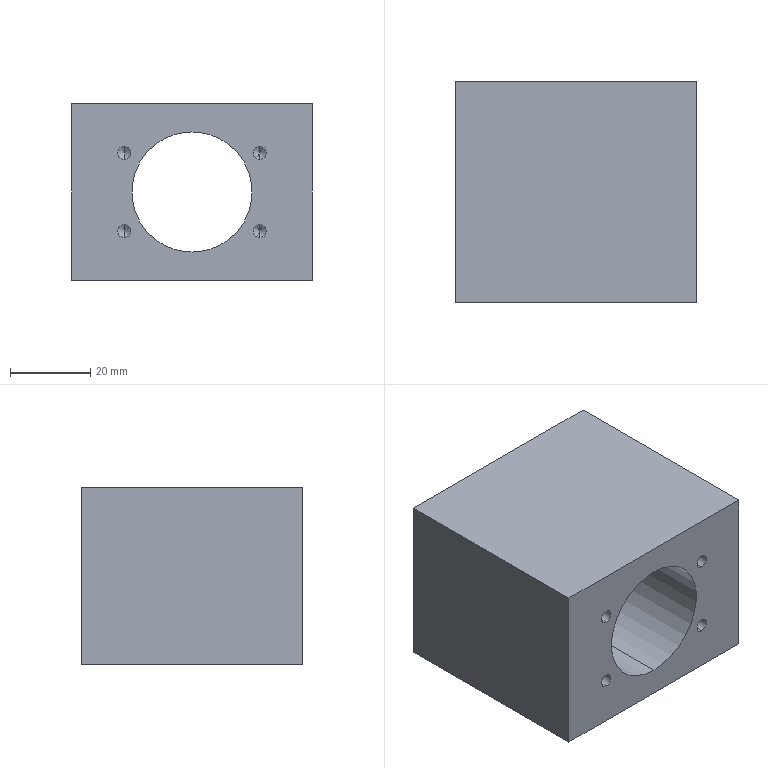Part | STEP file | X77-07003 | 1 solid | 40 faces | box 60 x 55 x 44 mm | volume 104749 mm3 | cylinder 18 | cone 16 | plane 6 | commonest cylinder face diameters 3.3 x8 5 x8 30 x2
STEP:
#1=CARTESIAN_POINT('',(18.182,-106.098,3.));
#2=VERTEX_POINT('',#1);
#3=CARTESIAN_POINT('',(13.182,-106.098,3.));
#4=VERTEX_POINT('',#3);
#5=CARTESIAN_POINT('',(15.682,-106.098,3.));
#6=DIRECTION('',(0.,0.,-1.));
#7=DIRECTION('',(-1.,0.,0.));
#8=AXIS2_PLACEMENT_3D('',#5,#6,#7);
#9=CIRCLE('',#8,2.5);
#10=EDGE_CURVE('',#2,#4,#9,.T.);
#11=ORIENTED_EDGE('',*,*,#10,.F.);
#12=CARTESIAN_POINT('',(18.182,-106.098,-12.));
#13=VERTEX_POINT('',#12);
#14=CARTESIAN_POINT('',(18.182,-106.098,-12.));
#15=DIRECTION('',(0.,0.,-1.));
#16=VECTOR('',#15,1000.);
#17=LINE('',#14,#16);
#18=EDGE_CURVE('',#2,#13,#17,.T.);
#19=ORIENTED_EDGE('',*,*,#18,.T.);
#20=CARTESIAN_POINT('',(13.182,-106.098,-12.));
#21=VERTEX_POINT('',#20);
#22=CARTESIAN_POINT('',(15.682,-106.098,-12.));
#23=DIRECTION('',(0.,0.,-1.));
#24=DIRECTION('',(-1.,0.,0.));
#25=AXIS2_PLACEMENT_3D('',#22,#23,#24);
#26=CIRCLE('',#25,2.5);
#27=EDGE_CURVE('',#13,#21,#26,.T.);
#28=ORIENTED_EDGE('',*,*,#27,.T.);
#29=CARTESIAN_POINT('',(13.182,-106.098,-12.));
#30=DIRECTION('',(0.,0.,-1.));
#31=VECTOR('',#30,1000.);
#32=LINE('',#29,#31);
#33=EDGE_CURVE('',#4,#21,#32,.T.);
#34=ORIENTED_EDGE('',*,*,#33,.F.);
#35=EDGE_LOOP('',(#11,#19,#28,#34));
#36=FACE_OUTER_BOUND('',#35,.T.);
#37=CARTESIAN_POINT('',(15.682,-106.098,-12.));
#38=DIRECTION('',(0.,0.,-1.));
#39=DIRECTION('',(-1.,0.,0.));
#40=AXIS2_PLACEMENT_3D('',#37,#38,#39);
#41=CYLINDRICAL_SURFACE('',#40,2.5);
#42=ADVANCED_FACE('',(#36),#41,.F.);
#43=CARTESIAN_POINT('',(15.682,-106.098,4.502));
#44=VERTEX_POINT('',#43);
#45=CARTESIAN_POINT('',(13.182,-106.098,3.));
#46=DIRECTION('',(-0.8572,0.,-0.515));
#47=VECTOR('',#46,1000.);
#48=LINE('',#45,#47);
#49=EDGE_CURVE('',#44,#4,#48,.T.);
#50=ORIENTED_EDGE('',*,*,#49,.F.);
#51=CARTESIAN_POINT('',(18.182,-106.098,3.));
#52=DIRECTION('',(0.8572,0.,-0.515));
#53=VECTOR('',#52,1000.);
#54=LINE('',#51,#53);
#55=EDGE_CURVE('',#44,#2,#54,.T.);
#56=ORIENTED_EDGE('',*,*,#55,.T.);
#57=ORIENTED_EDGE('',*,*,#10,.T.);
#58=EDGE_LOOP('',(#50,#56,#57));
#59=FACE_OUTER_BOUND('',#58,.T.);
#60=CARTESIAN_POINT('',(15.682,-106.098,3.));
#61=DIRECTION('',(0.,0.,-1.));
#62=DIRECTION('',(-1.,0.,0.));
#63=AXIS2_PLACEMENT_3D('',#60,#61,#62);
#64=CONICAL_SURFACE('',#63,2.5,1.03);
#65=ADVANCED_FACE('',(#59),#64,.F.);
#66=CARTESIAN_POINT('',(-26.818,-106.098,3.));
#67=VERTEX_POINT('',#66);
#68=CARTESIAN_POINT('',(-31.818,-106.098,3.));
#69=VERTEX_POINT('',#68);
#70=CARTESIAN_POINT('',(-29.318,-106.098,3.));
#71=DIRECTION('',(0.,0.,-1.));
#72=DIRECTION('',(-1.,0.,0.));
#73=AXIS2_PLACEMENT_3D('',#70,#71,#72);
#74=CIRCLE('',#73,2.5);
#75=EDGE_CURVE('',#67,#69,#74,.T.);
#76=ORIENTED_EDGE('',*,*,#75,.F.);
#77=CARTESIAN_POINT('',(-26.818,-106.098,-12.));
#78=VERTEX_POINT('',#77);
#79=CARTESIAN_POINT('',(-26.818,-106.098,-12.));
#80=DIRECTION('',(0.,0.,-1.));
#81=VECTOR('',#80,1000.);
#82=LINE('',#79,#81);
#83=EDGE_CURVE('',#67,#78,#82,.T.);
#84=ORIENTED_EDGE('',*,*,#83,.T.);
#85=CARTESIAN_POINT('',(-31.818,-106.098,-12.));
#86=VERTEX_POINT('',#85);
#87=CARTESIAN_POINT('',(-29.318,-106.098,-12.));
#88=DIRECTION('',(0.,0.,-1.));
#89=DIRECTION('',(-1.,0.,0.));
#90=AXIS2_PLACEMENT_3D('',#87,#88,#89);
#91=CIRCLE('',#90,2.5);
#92=EDGE_CURVE('',#78,#86,#91,.T.);
#93=ORIENTED_EDGE('',*,*,#92,.T.);
#94=CARTESIAN_POINT('',(-31.818,-106.098,-12.));
#95=DIRECTION('',(0.,0.,-1.));
#96=VECTOR('',#95,1000.);
#97=LINE('',#94,#96);
#98=EDGE_CURVE('',#69,#86,#97,.T.);
#99=ORIENTED_EDGE('',*,*,#98,.F.);
#100=EDGE_LOOP('',(#76,#84,#93,#99));
#101=FACE_OUTER_BOUND('',#100,.T.);
#102=CARTESIAN_POINT('',(-29.318,-106.098,-12.));
#103=DIRECTION('',(0.,0.,-1.));
#104=DIRECTION('',(-1.,0.,0.));
#105=AXIS2_PLACEMENT_3D('',#102,#103,#104);
#106=CYLINDRICAL_SURFACE('',#105,2.5);
#107=ADVANCED_FACE('',(#101),#106,.F.);
#108=CARTESIAN_POINT('',(-29.318,-106.098,4.502));
#109=VERTEX_POINT('',#108);
#110=CARTESIAN_POINT('',(-31.818,-106.098,3.));
#111=DIRECTION('',(-0.8572,0.,-0.515));
#112=VECTOR('',#111,1000.);
#113=LINE('',#110,#112);
#114=EDGE_CURVE('',#109,#69,#113,.T.);
#115=ORIENTED_EDGE('',*,*,#114,.F.);
#116=CARTESIAN_POINT('',(-26.818,-106.098,3.));
#117=DIRECTION('',(0.8572,0.,-0.515));
#118=VECTOR('',#117,1000.);
#119=LINE('',#116,#118);
#120=EDGE_CURVE('',#109,#67,#119,.T.);
#121=ORIENTED_EDGE('',*,*,#120,.T.);
#122=ORIENTED_EDGE('',*,*,#75,.T.);
#123=EDGE_LOOP('',(#115,#121,#122));
#124=FACE_OUTER_BOUND('',#123,.T.);
#125=CARTESIAN_POINT('',(-29.318,-106.098,3.));
#126=DIRECTION('',(0.,0.,-1.));
#127=DIRECTION('',(-1.,0.,0.));
#128=AXIS2_PLACEMENT_3D('',#125,#126,#127);
#129=CONICAL_SURFACE('',#128,2.5,1.03);
#130=ADVANCED_FACE('',(#124),#129,.F.);
#131=CARTESIAN_POINT('',(18.182,-146.098,3.));
#132=VERTEX_POINT('',#131);
#133=CARTESIAN_POINT('',(13.182,-146.098,3.));
#134=VERTEX_POINT('',#133);
#135=CARTESIAN_POINT('',(15.682,-146.098,3.));
#136=DIRECTION('',(0.,0.,-1.));
#137=DIRECTION('',(-1.,0.,0.));
#138=AXIS2_PLACEMENT_3D('',#135,#136,#137);
#139=CIRCLE('',#138,2.5);
#140=EDGE_CURVE('',#132,#134,#139,.T.);
#141=ORIENTED_EDGE('',*,*,#140,.F.);
#142=CARTESIAN_POINT('',(18.182,-146.098,-12.));
#143=VERTEX_POINT('',#142);
#144=CARTESIAN_POINT('',(18.182,-146.098,-12.));
#145=DIRECTION('',(0.,0.,-1.));
#146=VECTOR('',#145,1000.);
#147=LINE('',#144,#146);
#148=EDGE_CURVE('',#132,#143,#147,.T.);
#149=ORIENTED_EDGE('',*,*,#148,.T.);
#150=CARTESIAN_POINT('',(13.182,-146.098,-12.));
#151=VERTEX_POINT('',#150);
#152=CARTESIAN_POINT('',(15.682,-146.098,-12.));
#153=DIRECTION('',(0.,0.,-1.));
#154=DIRECTION('',(-1.,0.,0.));
#155=AXIS2_PLACEMENT_3D('',#152,#153,#154);
#156=CIRCLE('',#155,2.5);
#157=EDGE_CURVE('',#143,#151,#156,.T.);
#158=ORIENTED_EDGE('',*,*,#157,.T.);
#159=CARTESIAN_POINT('',(13.182,-146.098,-12.));
#160=DIRECTION('',(0.,0.,-1.));
#161=VECTOR('',#160,1000.);
#162=LINE('',#159,#161);
#163=EDGE_CURVE('',#134,#151,#162,.T.);
#164=ORIENTED_EDGE('',*,*,#163,.F.);
#165=EDGE_LOOP('',(#141,#149,#158,#164));
#166=FACE_OUTER_BOUND('',#165,.T.);
#167=CARTESIAN_POINT('',(15.682,-146.098,-12.));
#168=DIRECTION('',(0.,0.,-1.));
#169=DIRECTION('',(-1.,0.,0.));
#170=AXIS2_PLACEMENT_3D('',#167,#168,#169);
#171=CYLINDRICAL_SURFACE('',#170,2.5);
#172=ADVANCED_FACE('',(#166),#171,.F.);
#173=CARTESIAN_POINT('',(15.682,-146.098,4.502));
#174=VERTEX_POINT('',#173);
#175=CARTESIAN_POINT('',(13.182,-146.098,3.));
#176=DIRECTION('',(-0.8572,0.,-0.515));
#177=VECTOR('',#176,1000.);
#178=LINE('',#175,#177);
#179=EDGE_CURVE('',#174,#134,#178,.T.);
#180=ORIENTED_EDGE('',*,*,#179,.F.);
#181=CARTESIAN_POINT('',(18.182,-146.098,3.));
#182=DIRECTION('',(0.8572,0.,-0.515));
#183=VECTOR('',#182,1000.);
#184=LINE('',#181,#183);
#185=EDGE_CURVE('',#174,#132,#184,.T.);
#186=ORIENTED_EDGE('',*,*,#185,.T.);
#187=ORIENTED_EDGE('',*,*,#140,.T.);
#188=EDGE_LOOP('',(#180,#186,#187));
#189=FACE_OUTER_BOUND('',#188,.T.);
#190=CARTESIAN_POINT('',(15.682,-146.098,3.));
#191=DIRECTION('',(0.,0.,-1.));
#192=DIRECTION('',(-1.,0.,0.));
#193=AXIS2_PLACEMENT_3D('',#190,#191,#192);
#194=CONICAL_SURFACE('',#193,2.5,1.03);
#195=ADVANCED_FACE('',(#189),#194,.F.);
#196=CARTESIAN_POINT('',(-26.818,-146.098,3.));
#197=VERTEX_POINT('',#196);
#198=CARTESIAN_POINT('',(-31.818,-146.098,3.));
#199=VERTEX_POINT('',#198);
#200=CARTESIAN_POINT('',(-29.318,-146.098,3.));
#201=DIRECTION('',(0.,0.,-1.));
#202=DIRECTION('',(-1.,0.,0.));
#203=AXIS2_PLACEMENT_3D('',#200,#201,#202);
#204=CIRCLE('',#203,2.5);
#205=EDGE_CURVE('',#197,#199,#204,.T.);
#206=ORIENTED_EDGE('',*,*,#205,.F.);
#207=CARTESIAN_POINT('',(-26.818,-146.098,-12.));
#208=VERTEX_POINT('',#207);
#209=CARTESIAN_POINT('',(-26.818,-146.098,-12.));
#210=DIRECTION('',(0.,0.,-1.));
#211=VECTOR('',#210,1000.);
#212=LINE('',#209,#211);
#213=EDGE_CURVE('',#197,#208,#212,.T.);
#214=ORIENTED_EDGE('',*,*,#213,.T.);
#215=CARTESIAN_POINT('',(-31.818,-146.098,-12.));
#216=VERTEX_POINT('',#215);
#217=CARTESIAN_POINT('',(-29.318,-146.098,-12.));
#218=DIRECTION('',(0.,0.,-1.));
#219=DIRECTION('',(-1.,0.,0.));
#220=AXIS2_PLACEMENT_3D('',#217,#218,#219);
#221=CIRCLE('',#220,2.5);
#222=EDGE_CURVE('',#208,#216,#221,.T.);
#223=ORIENTED_EDGE('',*,*,#222,.T.);
#224=CARTESIAN_POINT('',(-31.818,-146.098,-12.));
#225=DIRECTION('',(0.,0.,-1.));
#226=VECTOR('',#225,1000.);
#227=LINE('',#224,#226);
#228=EDGE_CURVE('',#199,#216,#227,.T.);
#229=ORIENTED_EDGE('',*,*,#228,.F.);
#230=EDGE_LOOP('',(#206,#214,#223,#229));
#231=FACE_OUTER_BOUND('',#230,.T.);
#232=CARTESIAN_POINT('',(-29.318,-146.098,-12.));
#233=DIRECTION('',(0.,0.,-1.));
#234=DIRECTION('',(-1.,0.,0.));
#235=AXIS2_PLACEMENT_3D('',#232,#233,#234);
#236=CYLINDRICAL_SURFACE('',#235,2.5);
#237=ADVANCED_FACE('',(#231),#236,.F.);
#238=CARTESIAN_POINT('',(-29.318,-146.098,4.502));
#239=VERTEX_POINT('',#238);
#240=CARTESIAN_POINT('',(-31.818,-146.098,3.));
#241=DIRECTION('',(-0.8572,0.,-0.515));
#242=VECTOR('',#241,1000.);
#243=LINE('',#240,#242);
#244=EDGE_CURVE('',#239,#199,#243,.T.);
#245=ORIENTED_EDGE('',*,*,#244,.F.);
#246=CARTESIAN_POINT('',(-26.818,-146.098,3.));
#247=DIRECTION('',(0.8572,0.,-0.515));
#248=VECTOR('',#247,1000.);
#249=LINE('',#246,#248);
#250=EDGE_CURVE('',#239,#197,#249,.T.);
#251=ORIENTED_EDGE('',*,*,#250,.T.);
#252=ORIENTED_EDGE('',*,*,#205,.T.);
#253=EDGE_LOOP('',(#245,#251,#252));
#254=FACE_OUTER_BOUND('',#253,.T.);
#255=CARTESIAN_POINT('',(-29.318,-146.098,3.));
#256=DIRECTION('',(0.,0.,-1.));
#257=DIRECTION('',(-1.,0.,0.));
#258=AXIS2_PLACEMENT_3D('',#255,#256,#257);
#259=CONICAL_SURFACE('',#258,2.5,1.03);
#260=ADVANCED_FACE('',(#254),#259,.F.);
#261=CARTESIAN_POINT('',(-23.706,-143.498,21.4));
#262=VERTEX_POINT('',#261);
#263=CARTESIAN_POINT('',(-23.706,-143.498,18.1));
#264=VERTEX_POINT('',#263);
#265=CARTESIAN_POINT('',(-23.706,-143.498,19.75));
#266=DIRECTION('',(0.,-1.,0.));
#267=DIRECTION('',(0.,0.,-1.));
#268=AXIS2_PLACEMENT_3D('',#265,#266,#267);
#269=CIRCLE('',#268,1.65);
#270=EDGE_CURVE('',#262,#264,#269,.T.);
#271=ORIENTED_EDGE('',*,*,#270,.F.);
#272=CARTESIAN_POINT('',(-23.706,-153.598,21.4));
#273=VERTEX_POINT('',#272);
#274=CARTESIAN_POINT('',(-23.706,-153.598,21.4));
#275=DIRECTION('',(0.,-1.,0.));
#276=VECTOR('',#275,1000.);
#277=LINE('',#274,#276);
#278=EDGE_CURVE('',#262,#273,#277,.T.);
#279=ORIENTED_EDGE('',*,*,#278,.T.);
#280=CARTESIAN_POINT('',(-23.706,-153.598,18.1));
#281=VERTEX_POINT('',#280);
#282=CARTESIAN_POINT('',(-23.706,-153.598,19.75));
#283=DIRECTION('',(0.,-1.,0.));
#284=DIRECTION('',(0.,0.,-1.));
#285=AXIS2_PLACEMENT_3D('',#282,#283,#284);
#286=CIRCLE('',#285,1.65);
#287=EDGE_CURVE('',#273,#281,#286,.T.);
#288=ORIENTED_EDGE('',*,*,#287,.T.);
#289=CARTESIAN_POINT('',(-23.706,-153.598,18.1));
#290=DIRECTION('',(0.,-1.,0.));
#291=VECTOR('',#290,1000.);
#292=LINE('',#289,#291);
#293=EDGE_CURVE('',#264,#281,#292,.T.);
#294=ORIENTED_EDGE('',*,*,#293,.F.);
#295=EDGE_LOOP('',(#271,#279,#288,#294));
#296=FACE_OUTER_BOUND('',#295,.T.);
#297=CARTESIAN_POINT('',(-23.706,-153.598,19.75));
#298=DIRECTION('',(0.,-1.,0.));
#299=DIRECTION('',(0.,0.,-1.));
#300=AXIS2_PLACEMENT_3D('',#297,#298,#299);
#301=CYLINDRICAL_SURFACE('',#300,1.65);
#302=ADVANCED_FACE('',(#296),#301,.F.);
#303=CARTESIAN_POINT('',(-23.706,-142.506,19.75));
#304=VERTEX_POINT('',#303);
#305=CARTESIAN_POINT('',(-23.706,-143.498,18.1));
#306=DIRECTION('',(0.,-0.515,-0.8572));
#307=VECTOR('',#306,1000.);
#308=LINE('',#305,#307);
#309=EDGE_CURVE('',#304,#264,#308,.T.);
#310=ORIENTED_EDGE('',*,*,#309,.F.);
#311=CARTESIAN_POINT('',(-23.706,-143.498,21.4));
#312=DIRECTION('',(0.,-0.515,0.8572));
#313=VECTOR('',#312,1000.);
#314=LINE('',#311,#313);
#315=EDGE_CURVE('',#304,#262,#314,.T.);
#316=ORIENTED_EDGE('',*,*,#315,.T.);
#317=ORIENTED_EDGE('',*,*,#270,.T.);
#318=EDGE_LOOP('',(#310,#316,#317));
#319=FACE_OUTER_BOUND('',#318,.T.);
#320=CARTESIAN_POINT('',(-23.706,-143.498,19.75));
#321=DIRECTION('',(0.,-1.,0.));
#322=DIRECTION('',(0.,0.,-1.));
#323=AXIS2_PLACEMENT_3D('',#320,#321,#322);
#324=CONICAL_SURFACE('',#323,1.65,1.03);
#325=ADVANCED_FACE('',(#319),#324,.F.);
#326=CARTESIAN_POINT('',(-23.706,-143.498,1.9));
#327=VERTEX_POINT('',#326);
#328=CARTESIAN_POINT('',(-23.706,-143.498,-1.4));
#329=VERTEX_POINT('',#328);
#330=CARTESIAN_POINT('',(-23.706,-143.498,0.25));
#331=DIRECTION('',(0.,-1.,0.));
#332=DIRECTION('',(0.,0.,-1.));
#333=AXIS2_PLACEMENT_3D('',#330,#331,#332);
#334=CIRCLE('',#333,1.65);
#335=EDGE_CURVE('',#327,#329,#334,.T.);
#336=ORIENTED_EDGE('',*,*,#335,.F.);
#337=CARTESIAN_POINT('',(-23.706,-153.598,1.9));
#338=VERTEX_POINT('',#337);
#339=CARTESIAN_POINT('',(-23.706,-153.598,1.9));
#340=DIRECTION('',(0.,-1.,0.));
#341=VECTOR('',#340,1000.);
#342=LINE('',#339,#341);
#343=EDGE_CURVE('',#327,#338,#342,.T.);
#344=ORIENTED_EDGE('',*,*,#343,.T.);
#345=CARTESIAN_POINT('',(-23.706,-153.598,-1.4));
#346=VERTEX_POINT('',#345);
#347=CARTESIAN_POINT('',(-23.706,-153.598,0.25));
#348=DIRECTION('',(0.,-1.,0.));
#349=DIRECTION('',(0.,0.,-1.));
#350=AXIS2_PLACEMENT_3D('',#347,#348,#349);
#351=CIRCLE('',#350,1.65);
#352=EDGE_CURVE('',#338,#346,#351,.T.);
#353=ORIENTED_EDGE('',*,*,#352,.T.);
#354=CARTESIAN_POINT('',(-23.706,-153.598,-1.4));
#355=DIRECTION('',(0.,-1.,0.));
#356=VECTOR('',#355,1000.);
#357=LINE('',#354,#356);
#358=EDGE_CURVE('',#329,#346,#357,.T.);
#359=ORIENTED_EDGE('',*,*,#358,.F.);
#360=EDGE_LOOP('',(#336,#344,#353,#359));
#361=FACE_OUTER_BOUND('',#360,.T.);
#362=CARTESIAN_POINT('',(-23.706,-153.598,0.25));
#363=DIRECTION('',(0.,-1.,0.));
#364=DIRECTION('',(0.,0.,-1.));
#365=AXIS2_PLACEMENT_3D('',#362,#363,#364);
#366=CYLINDRICAL_SURFACE('',#365,1.65);
#367=ADVANCED_FACE('',(#361),#366,.F.);
#368=CARTESIAN_POINT('',(-23.706,-142.506,0.25));
#369=VERTEX_POINT('',#368);
#370=CARTESIAN_POINT('',(-23.706,-143.498,-1.4));
#371=DIRECTION('',(0.,-0.515,-0.8572));
#372=VECTOR('',#371,1000.);
#373=LINE('',#370,#372);
#374=EDGE_CURVE('',#369,#329,#373,.T.);
#375=ORIENTED_EDGE('',*,*,#374,.F.);
#376=CARTESIAN_POINT('',(-23.706,-143.498,1.9));
#377=DIRECTION('',(0.,-0.515,0.8572));
#378=VECTOR('',#377,1000.);
#379=LINE('',#376,#378);
#380=EDGE_CURVE('',#369,#327,#379,.T.);
#381=ORIENTED_EDGE('',*,*,#380,.T.);
#382=ORIENTED_EDGE('',*,*,#335,.T.);
#383=EDGE_LOOP('',(#375,#381,#382));
#384=FACE_OUTER_BOUND('',#383,.T.);
#385=CARTESIAN_POINT('',(-23.706,-143.498,0.25));
#386=DIRECTION('',(0.,-1.,0.));
#387=DIRECTION('',(0.,0.,-1.));
#388=AXIS2_PLACEMENT_3D('',#385,#386,#387);
#389=CONICAL_SURFACE('',#388,1.65,1.03);
#390=ADVANCED_FACE('',(#384),#389,.F.);
#391=CARTESIAN_POINT('',(10.069,-143.498,1.9));
#392=VERTEX_POINT('',#391);
#393=CARTESIAN_POINT('',(10.069,-143.498,-1.4));
#394=VERTEX_POINT('',#393);
#395=CARTESIAN_POINT('',(10.069,-143.498,0.25));
#396=DIRECTION('',(0.,-1.,0.));
#397=DIRECTION('',(0.,0.,-1.));
#398=AXIS2_PLACEMENT_3D('',#395,#396,#397);
#399=CIRCLE('',#398,1.65);
#400=EDGE_CURVE('',#392,#394,#399,.T.);
#401=ORIENTED_EDGE('',*,*,#400,.F.);
#402=CARTESIAN_POINT('',(10.069,-153.598,1.9));
#403=VERTEX_POINT('',#402);
#404=CARTESIAN_POINT('',(10.069,-153.598,1.9));
#405=DIRECTION('',(0.,-1.,0.));
#406=VECTOR('',#405,1000.);
#407=LINE('',#404,#406);
#408=EDGE_CURVE('',#392,#403,#407,.T.);
#409=ORIENTED_EDGE('',*,*,#408,.T.);
#410=CARTESIAN_POINT('',(10.069,-153.598,-1.4));
#411=VERTEX_POINT('',#410);
#412=CARTESIAN_POINT('',(10.069,-153.598,0.25));
#413=DIRECTION('',(0.,-1.,0.));
#414=DIRECTION('',(0.,0.,-1.));
#415=AXIS2_PLACEMENT_3D('',#412,#413,#414);
#416=CIRCLE('',#415,1.65);
#417=EDGE_CURVE('',#403,#411,#416,.T.);
#418=ORIENTED_EDGE('',*,*,#417,.T.);
#419=CARTESIAN_POINT('',(10.069,-153.598,-1.4));
#420=DIRECTION('',(0.,-1.,0.));
#421=VECTOR('',#420,1000.);
#422=LINE('',#419,#421);
#423=EDGE_CURVE('',#394,#411,#422,.T.);
#424=ORIENTED_EDGE('',*,*,#423,.F.);
#425=EDGE_LOOP('',(#401,#409,#418,#424));
#426=FACE_OUTER_BOUND('',#425,.T.);
#427=CARTESIAN_POINT('',(10.069,-153.598,0.25));
#428=DIRECTION('',(0.,-1.,0.));
#429=DIRECTION('',(0.,0.,-1.));
#430=AXIS2_PLACEMENT_3D('',#427,#428,#429);
#431=CYLINDRICAL_SURFACE('',#430,1.65);
#432=ADVANCED_FACE('',(#426),#431,.F.);
#433=CARTESIAN_POINT('',(10.069,-142.506,0.25));
#434=VERTEX_POINT('',#433);
#435=CARTESIAN_POINT('',(10.069,-143.498,-1.4));
#436=DIRECTION('',(0.,-0.515,-0.8572));
#437=VECTOR('',#436,1000.);
#438=LINE('',#435,#437);
#439=EDGE_CURVE('',#434,#394,#438,.T.);
#440=ORIENTED_EDGE('',*,*,#439,.F.);
#441=CARTESIAN_POINT('',(10.069,-143.498,1.9));
#442=DIRECTION('',(0.,-0.515,0.8572));
#443=VECTOR('',#442,1000.);
#444=LINE('',#441,#443);
#445=EDGE_CURVE('',#434,#392,#444,.T.);
#446=ORIENTED_EDGE('',*,*,#445,.T.);
#447=ORIENTED_EDGE('',*,*,#400,.T.);
#448=EDGE_LOOP('',(#440,#446,#447));
#449=FACE_OUTER_BOUND('',#448,.T.);
#450=CARTESIAN_POINT('',(10.069,-143.498,0.25));
#451=DIRECTION('',(0.,-1.,0.));
#452=DIRECTION('',(0.,0.,-1.));
#453=AXIS2_PLACEMENT_3D('',#450,#451,#452);
#454=CONICAL_SURFACE('',#453,1.65,1.03);
#455=ADVANCED_FACE('',(#449),#454,.F.);
#456=CARTESIAN_POINT('',(10.069,-143.498,21.4));
#457=VERTEX_POINT('',#456);
#458=CARTESIAN_POINT('',(10.069,-143.498,18.1));
#459=VERTEX_POINT('',#458);
#460=CARTESIAN_POINT('',(10.069,-143.498,19.75));
#461=DIRECTION('',(0.,-1.,0.));
#462=DIRECTION('',(0.,0.,-1.));
#463=AXIS2_PLACEMENT_3D('',#460,#461,#462);
#464=CIRCLE('',#463,1.65);
#465=EDGE_CURVE('',#457,#459,#464,.T.);
#466=ORIENTED_EDGE('',*,*,#465,.F.);
#467=CARTESIAN_POINT('',(10.069,-153.598,21.4));
#468=VERTEX_POINT('',#467);
#469=CARTESIAN_POINT('',(10.069,-153.598,21.4));
#470=DIRECTION('',(0.,-1.,0.));
#471=VECTOR('',#470,1000.);
#472=LINE('',#469,#471);
#473=EDGE_CURVE('',#457,#468,#472,.T.);
#474=ORIENTED_EDGE('',*,*,#473,.T.);
#475=CARTESIAN_POINT('',(10.069,-153.598,18.1));
#476=VERTEX_POINT('',#475);
#477=CARTESIAN_POINT('',(10.069,-153.598,19.75));
#478=DIRECTION('',(0.,-1.,0.));
#479=DIRECTION('',(0.,0.,-1.));
#480=AXIS2_PLACEMENT_3D('',#477,#478,#479);
#481=CIRCLE('',#480,1.65);
#482=EDGE_CURVE('',#468,#476,#481,.T.);
#483=ORIENTED_EDGE('',*,*,#482,.T.);
#484=CARTESIAN_POINT('',(10.069,-153.598,18.1));
#485=DIRECTION('',(0.,-1.,0.));
#486=VECTOR('',#485,1000.);
#487=LINE('',#484,#486);
#488=EDGE_CURVE('',#459,#476,#487,.T.);
#489=ORIENTED_EDGE('',*,*,#488,.F.);
#490=EDGE_LOOP('',(#466,#474,#483,#489));
#491=FACE_OUTER_BOUND('',#490,.T.);
#492=CARTESIAN_POINT('',(10.069,-153.598,19.75));
#493=DIRECTION('',(0.,-1.,0.));
#494=DIRECTION('',(0.,0.,-1.));
#495=AXIS2_PLACEMENT_3D('',#492,#493,#494);
#496=CYLINDRICAL_SURFACE('',#495,1.65);
#497=ADVANCED_FACE('',(#491),#496,.F.);
#498=CARTESIAN_POINT('',(10.069,-142.506,19.75));
#499=VERTEX_POINT('',#498);
#500=CARTESIAN_POINT('',(10.069,-143.498,18.1));
#501=DIRECTION('',(0.,-0.515,-0.8572));
#502=VECTOR('',#501,1000.);
#503=LINE('',#500,#502);
#504=EDGE_CURVE('',#499,#459,#503,.T.);
#505=ORIENTED_EDGE('',*,*,#504,.F.);
#506=CARTESIAN_POINT('',(10.069,-143.498,21.4));
#507=DIRECTION('',(0.,-0.515,0.8572));
#508=VECTOR('',#507,1000.);
#509=LINE('',#506,#508);
#510=EDGE_CURVE('',#499,#457,#509,.T.);
#511=ORIENTED_EDGE('',*,*,#510,.T.);
#512=ORIENTED_EDGE('',*,*,#465,.T.);
#513=EDGE_LOOP('',(#505,#511,#512));
#514=FACE_OUTER_BOUND('',#513,.T.);
#515=CARTESIAN_POINT('',(10.069,-143.498,19.75));
#516=DIRECTION('',(0.,-1.,0.));
#517=DIRECTION('',(0.,0.,-1.));
#518=AXIS2_PLACEMENT_3D('',#515,#516,#517);
#519=CONICAL_SURFACE('',#518,1.65,1.03);
#520=ADVANCED_FACE('',(#514),#519,.F.);
#521=CARTESIAN_POINT('',(-6.818,-153.598,-5.));
#522=VERTEX_POINT('',#521);
#523=CARTESIAN_POINT('',(-6.818,-153.598,25.));
#524=VERTEX_POINT('',#523);
#525=CARTESIAN_POINT('',(-6.818,-153.598,10.));
#526=DIRECTION('',(0.,1.,0.));
#527=DIRECTION('',(0.,0.,1.));
#528=AXIS2_PLACEMENT_3D('',#525,#526,#527);
#529=CIRCLE('',#528,15.);
#530=EDGE_CURVE('',#522,#524,#529,.T.);
#531=ORIENTED_EDGE('',*,*,#530,.F.);
#532=CARTESIAN_POINT('',(-6.818,-98.598,-5.));
#533=VERTEX_POINT('',#532);
#534=CARTESIAN_POINT('',(-6.818,-153.598,-5.));
#535=DIRECTION('',(0.,1.,0.));
#536=VECTOR('',#535,1000.);
#537=LINE('',#534,#536);
#538=EDGE_CURVE('',#522,#533,#537,.T.);
#539=ORIENTED_EDGE('',*,*,#538,.T.);
#540=CARTESIAN_POINT('',(-6.818,-98.598,25.));
#541=VERTEX_POINT('',#540);
#542=CARTESIAN_POINT('',(-6.818,-98.598,10.));
#543=DIRECTION('',(0.,1.,0.));
#544=DIRECTION('',(0.,0.,1.));
#545=AXIS2_PLACEMENT_3D('',#542,#543,#544);
#546=CIRCLE('',#545,15.);
#547=EDGE_CURVE('',#533,#541,#546,.T.);
#548=ORIENTED_EDGE('',*,*,#547,.T.);
#549=CARTESIAN_POINT('',(-6.818,-153.598,25.));
#550=DIRECTION('',(0.,1.,0.));
#551=VECTOR('',#550,1000.);
#552=LINE('',#549,#551);
#553=EDGE_CURVE('',#524,#541,#552,.T.);
#554=ORIENTED_EDGE('',*,*,#553,.F.);
#555=EDGE_LOOP('',(#531,#539,#548,#554));
#556=FACE_OUTER_BOUND('',#555,.T.);
#557=CARTESIAN_POINT('',(-6.818,-153.598,10.));
#558=DIRECTION('',(0.,1.,0.));
#559=DIRECTION('',(0.,0.,1.));
#560=AXIS2_PLACEMENT_3D('',#557,#558,#559);
#561=CYLINDRICAL_SURFACE('',#560,15.);
#562=ADVANCED_FACE('',(#556),#561,.F.);
#563=CARTESIAN_POINT('',(-36.818,-98.598,32.));
#564=VERTEX_POINT('',#563);
#565=CARTESIAN_POINT('',(-36.818,-98.598,-12.));
#566=VERTEX_POINT('',#565);
#567=CARTESIAN_POINT('',(-36.818,-98.598,32.));
#568=DIRECTION('',(0.,0.,-1.));
#569=VECTOR('',#568,1000.);
#570=LINE('',#567,#569);
#571=EDGE_CURVE('',#564,#566,#570,.T.);
#572=ORIENTED_EDGE('',*,*,#571,.T.);
#573=CARTESIAN_POINT('',(-36.818,-153.598,-12.));
#574=VERTEX_POINT('',#573);
#575=CARTESIAN_POINT('',(-36.818,-153.598,-12.));
#576=DIRECTION('',(0.,1.,0.));
#577=VECTOR('',#576,1000.);
#578=LINE('',#575,#577);
#579=EDGE_CURVE('',#574,#566,#578,.T.);
#580=ORIENTED_EDGE('',*,*,#579,.F.);
#581=CARTESIAN_POINT('',(-36.818,-153.598,32.));
#582=VERTEX_POINT('',#581);
#583=CARTESIAN_POINT('',(-36.818,-153.598,32.));
#584=DIRECTION('',(0.,0.,-1.));
#585=VECTOR('',#584,1000.);
#586=LINE('',#583,#585);
#587=EDGE_CURVE('',#582,#574,#586,.T.);
#588=ORIENTED_EDGE('',*,*,#587,.F.);
#589=CARTESIAN_POINT('',(-36.818,-98.598,32.));
#590=DIRECTION('',(0.,-1.,0.));
#591=VECTOR('',#590,1000.);
#592=LINE('',#589,#591);
#593=EDGE_CURVE('',#564,#582,#592,.T.);
#594=ORIENTED_EDGE('',*,*,#593,.F.);
#595=EDGE_LOOP('',(#572,#580,#588,#594));
#596=FACE_OUTER_BOUND('',#595,.T.);
#597=CARTESIAN_POINT('',(-36.818,-98.598,32.));
#598=DIRECTION('',(1.,0.,0.));
#599=DIRECTION('',(0.,1.,0.));
#600=AXIS2_PLACEMENT_3D('',#597,#598,#599);
#601=PLANE('',#600);
#602=ADVANCED_FACE('',(#596),#601,.F.);
#603=CARTESIAN_POINT('',(-23.706,-153.598,19.75));
#604=DIRECTION('',(0.,-1.,0.));
#605=DIRECTION('',(0.,0.,-1.));
#606=AXIS2_PLACEMENT_3D('',#603,#604,#605);
#607=CIRCLE('',#606,1.65);
#608=EDGE_CURVE('',#281,#273,#607,.T.);
#609=ORIENTED_EDGE('',*,*,#608,.F.);
#610=ORIENTED_EDGE('',*,*,#287,.F.);
#611=EDGE_LOOP('',(#609,#610));
#612=FACE_BOUND('',#611,.T.);
#613=CARTESIAN_POINT('',(-23.706,-153.598,0.25));
#614=DIRECTION('',(0.,-1.,0.));
#615=DIRECTION('',(0.,0.,-1.));
#616=AXIS2_PLACEMENT_3D('',#613,#614,#615);
#617=CIRCLE('',#616,1.65);
#618=EDGE_CURVE('',#346,#338,#617,.T.);
#619=ORIENTED_EDGE('',*,*,#618,.F.);
#620=ORIENTED_EDGE('',*,*,#352,.F.);
#621=EDGE_LOOP('',(#619,#620));
#622=FACE_BOUND('',#621,.T.);
#623=CARTESIAN_POINT('',(10.069,-153.598,0.25));
#624=DIRECTION('',(0.,-1.,0.));
#625=DIRECTION('',(0.,0.,-1.));
#626=AXIS2_PLACEMENT_3D('',#623,#624,#625);
#627=CIRCLE('',#626,1.65);
#628=EDGE_CURVE('',#411,#403,#627,.T.);
#629=ORIENTED_EDGE('',*,*,#628,.F.);
#630=ORIENTED_EDGE('',*,*,#417,.F.);
#631=EDGE_LOOP('',(#629,#630));
#632=FACE_BOUND('',#631,.T.);
#633=CARTESIAN_POINT('',(10.069,-153.598,19.75));
#634=DIRECTION('',(0.,-1.,0.));
#635=DIRECTION('',(0.,0.,-1.));
#636=AXIS2_PLACEMENT_3D('',#633,#634,#635);
#637=CIRCLE('',#636,1.65);
#638=EDGE_CURVE('',#476,#468,#637,.T.);
#639=ORIENTED_EDGE('',*,*,#638,.F.);
#640=ORIENTED_EDGE('',*,*,#482,.F.);
#641=EDGE_LOOP('',(#639,#640));
#642=FACE_BOUND('',#641,.T.);
#643=CARTESIAN_POINT('',(-6.818,-153.598,10.));
#644=DIRECTION('',(0.,1.,0.));
#645=DIRECTION('',(0.,0.,1.));
#646=AXIS2_PLACEMENT_3D('',#643,#644,#645);
#647=CIRCLE('',#646,15.);
#648=EDGE_CURVE('',#524,#522,#647,.T.);
#649=ORIENTED_EDGE('',*,*,#648,.T.);
#650=ORIENTED_EDGE('',*,*,#530,.T.);
#651=EDGE_LOOP('',(#649,#650));
#652=FACE_BOUND('',#651,.T.);
#653=ORIENTED_EDGE('',*,*,#587,.T.);
#654=CARTESIAN_POINT('',(23.182,-153.598,-12.));
#655=VERTEX_POINT('',#654);
#656=CARTESIAN_POINT('',(23.182,-153.598,-12.));
#657=DIRECTION('',(-1.,0.,0.));
#658=VECTOR('',#657,1000.);
#659=LINE('',#656,#658);
#660=EDGE_CURVE('',#655,#574,#659,.T.);
#661=ORIENTED_EDGE('',*,*,#660,.F.);
#662=CARTESIAN_POINT('',(23.182,-153.598,32.));
#663=VERTEX_POINT('',#662);
#664=CARTESIAN_POINT('',(23.182,-153.598,32.));
#665=DIRECTION('',(0.,0.,-1.));
#666=VECTOR('',#665,1000.);
#667=LINE('',#664,#666);
#668=EDGE_CURVE('',#663,#655,#667,.T.);
#669=ORIENTED_EDGE('',*,*,#668,.F.);
#670=CARTESIAN_POINT('',(-36.818,-153.598,32.));
#671=DIRECTION('',(1.,0.,0.));
#672=VECTOR('',#671,1000.);
#673=LINE('',#670,#672);
#674=EDGE_CURVE('',#582,#663,#673,.T.);
#675=ORIENTED_EDGE('',*,*,#674,.F.);
#676=EDGE_LOOP('',(#653,#661,#669,#675));
#677=FACE_OUTER_BOUND('',#676,.T.);
#678=CARTESIAN_POINT('',(-36.818,-153.598,32.));
#679=DIRECTION('',(0.,1.,0.));
#680=DIRECTION('',(0.,0.,1.));
#681=AXIS2_PLACEMENT_3D('',#678,#679,#680);
#682=PLANE('',#681);
#683=ADVANCED_FACE('',(#612,#622,#632,#642,#652,#677),#682,.F.);
#684=ORIENTED_EDGE('',*,*,#668,.T.);
#685=CARTESIAN_POINT('',(23.182,-98.598,-12.));
#686=VERTEX_POINT('',#685);
#687=CARTESIAN_POINT('',(23.182,-153.598,-12.));
#688=DIRECTION('',(0.,-1.,0.));
#689=VECTOR('',#688,1000.);
#690=LINE('',#687,#689);
#691=EDGE_CURVE('',#686,#655,#690,.T.);
#692=ORIENTED_EDGE('',*,*,#691,.F.);
#693=CARTESIAN_POINT('',(23.182,-98.598,32.));
#694=VERTEX_POINT('',#693);
#695=CARTESIAN_POINT('',(23.182,-98.598,32.));
#696=DIRECTION('',(0.,0.,-1.));
#697=VECTOR('',#696,1000.);
#698=LINE('',#695,#697);
#699=EDGE_CURVE('',#694,#686,#698,.T.);
#700=ORIENTED_EDGE('',*,*,#699,.F.);
#701=CARTESIAN_POINT('',(23.182,-98.598,32.));
#702=DIRECTION('',(0.,1.,0.));
#703=VECTOR('',#702,1000.);
#704=LINE('',#701,#703);
#705=EDGE_CURVE('',#663,#694,#704,.T.);
#706=ORIENTED_EDGE('',*,*,#705,.F.);
#707=EDGE_LOOP('',(#684,#692,#700,#706));
#708=FACE_OUTER_BOUND('',#707,.T.);
#709=CARTESIAN_POINT('',(23.182,-98.598,32.));
#710=DIRECTION('',(-1.,0.,0.));
#711=DIRECTION('',(0.,-1.,0.));
#712=AXIS2_PLACEMENT_3D('',#709,#710,#711);
#713=PLANE('',#712);
#714=ADVANCED_FACE('',(#708),#713,.F.);
#715=CARTESIAN_POINT('',(-6.818,-98.598,10.));
#716=DIRECTION('',(0.,1.,0.));
#717=DIRECTION('',(0.,0.,1.));
#718=AXIS2_PLACEMENT_3D('',#715,#716,#717);
#719=CIRCLE('',#718,15.);
#720=EDGE_CURVE('',#541,#533,#719,.T.);
#721=ORIENTED_EDGE('',*,*,#720,.F.);
#722=ORIENTED_EDGE('',*,*,#547,.F.);
#723=EDGE_LOOP('',(#721,#722));
#724=FACE_BOUND('',#723,.T.);
#725=ORIENTED_EDGE('',*,*,#699,.T.);
#726=CARTESIAN_POINT('',(23.182,-98.598,-12.));
#727=DIRECTION('',(1.,0.,0.));
#728=VECTOR('',#727,1000.);
#729=LINE('',#726,#728);
#730=EDGE_CURVE('',#566,#686,#729,.T.);
#731=ORIENTED_EDGE('',*,*,#730,.F.);
#732=ORIENTED_EDGE('',*,*,#571,.F.);
#733=CARTESIAN_POINT('',(-36.818,-98.598,32.));
#734=DIRECTION('',(-1.,0.,0.));
#735=VECTOR('',#734,1000.);
#736=LINE('',#733,#735);
#737=EDGE_CURVE('',#694,#564,#736,.T.);
#738=ORIENTED_EDGE('',*,*,#737,.F.);
#739=EDGE_LOOP('',(#725,#731,#732,#738));
#740=FACE_OUTER_BOUND('',#739,.T.);
#741=CARTESIAN_POINT('',(-36.818,-98.598,32.));
#742=DIRECTION('',(0.,-1.,0.));
#743=DIRECTION('',(0.,0.,-1.));
#744=AXIS2_PLACEMENT_3D('',#741,#742,#743);
#745=PLANE('',#744);
#746=ADVANCED_FACE('',(#724,#740),#745,.F.);
#747=ORIENTED_EDGE('',*,*,#593,.T.);
#748=ORIENTED_EDGE('',*,*,#674,.T.);
#749=ORIENTED_EDGE('',*,*,#705,.T.);
#750=ORIENTED_EDGE('',*,*,#737,.T.);
#751=EDGE_LOOP('',(#747,#748,#749,#750));
#752=FACE_OUTER_BOUND('',#751,.T.);
#753=CARTESIAN_POINT('',(-36.818,-153.598,32.));
#754=DIRECTION('',(0.,0.,1.));
#755=DIRECTION('',(1.,0.,0.));
#756=AXIS2_PLACEMENT_3D('',#753,#754,#755);
#757=PLANE('',#756);
#758=ADVANCED_FACE('',(#752),#757,.T.);
#759=CARTESIAN_POINT('',(15.682,-106.098,-12.));
#760=DIRECTION('',(0.,0.,-1.));
#761=DIRECTION('',(-1.,0.,0.));
#762=AXIS2_PLACEMENT_3D('',#759,#760,#761);
#763=CIRCLE('',#762,2.5);
#764=EDGE_CURVE('',#21,#13,#763,.T.);
#765=ORIENTED_EDGE('',*,*,#764,.F.);
#766=ORIENTED_EDGE('',*,*,#27,.F.);
#767=EDGE_LOOP('',(#765,#766));
#768=FACE_BOUND('',#767,.T.);
#769=CARTESIAN_POINT('',(-29.318,-106.098,-12.));
#770=DIRECTION('',(0.,0.,-1.));
#771=DIRECTION('',(-1.,0.,0.));
#772=AXIS2_PLACEMENT_3D('',#769,#770,#771);
#773=CIRCLE('',#772,2.5);
#774=EDGE_CURVE('',#86,#78,#773,.T.);
#775=ORIENTED_EDGE('',*,*,#774,.F.);
#776=ORIENTED_EDGE('',*,*,#92,.F.);
#777=EDGE_LOOP('',(#775,#776));
#778=FACE_BOUND('',#777,.T.);
#779=CARTESIAN_POINT('',(15.682,-146.098,-12.));
#780=DIRECTION('',(0.,0.,-1.));
#781=DIRECTION('',(-1.,0.,0.));
#782=AXIS2_PLACEMENT_3D('',#779,#780,#781);
#783=CIRCLE('',#782,2.5);
#784=EDGE_CURVE('',#151,#143,#783,.T.);
#785=ORIENTED_EDGE('',*,*,#784,.F.);
#786=ORIENTED_EDGE('',*,*,#157,.F.);
#787=EDGE_LOOP('',(#785,#786));
#788=FACE_BOUND('',#787,.T.);
#789=CARTESIAN_POINT('',(-29.318,-146.098,-12.));
#790=DIRECTION('',(0.,0.,-1.));
#791=DIRECTION('',(-1.,0.,0.));
#792=AXIS2_PLACEMENT_3D('',#789,#790,#791);
#793=CIRCLE('',#792,2.5);
#794=EDGE_CURVE('',#216,#208,#793,.T.);
#795=ORIENTED_EDGE('',*,*,#794,.F.);
#796=ORIENTED_EDGE('',*,*,#222,.F.);
#797=EDGE_LOOP('',(#795,#796));
#798=FACE_BOUND('',#797,.T.);
#799=ORIENTED_EDGE('',*,*,#691,.T.);
#800=ORIENTED_EDGE('',*,*,#660,.T.);
#801=ORIENTED_EDGE('',*,*,#579,.T.);
#802=ORIENTED_EDGE('',*,*,#730,.T.);
#803=EDGE_LOOP('',(#799,#800,#801,#802));
#804=FACE_OUTER_BOUND('',#803,.T.);
#805=CARTESIAN_POINT('',(23.182,-98.598,-12.));
#806=DIRECTION('',(0.,0.,1.));
#807=DIRECTION('',(1.,0.,0.));
#808=AXIS2_PLACEMENT_3D('',#805,#806,#807);
#809=PLANE('',#808);
#810=ADVANCED_FACE('',(#768,#778,#788,#798,#804),#809,.F.);
#811=ORIENTED_EDGE('',*,*,#538,.F.);
#812=ORIENTED_EDGE('',*,*,#648,.F.);
#813=ORIENTED_EDGE('',*,*,#553,.T.);
#814=ORIENTED_EDGE('',*,*,#720,.T.);
#815=EDGE_LOOP('',(#811,#812,#813,#814));
#816=FACE_OUTER_BOUND('',#815,.T.);
#817=CARTESIAN_POINT('',(-6.818,-153.598,10.));
#818=DIRECTION('',(0.,1.,0.));
#819=DIRECTION('',(0.,0.,1.));
#820=AXIS2_PLACEMENT_3D('',#817,#818,#819);
#821=CYLINDRICAL_SURFACE('',#820,15.);
#822=ADVANCED_FACE('',(#816),#821,.F.);
#823=ORIENTED_EDGE('',*,*,#510,.F.);
#824=ORIENTED_EDGE('',*,*,#504,.T.);
#825=CARTESIAN_POINT('',(10.069,-143.498,19.75));
#826=DIRECTION('',(0.,-1.,0.));
#827=DIRECTION('',(0.,0.,-1.));
#828=AXIS2_PLACEMENT_3D('',#825,#826,#827);
#829=CIRCLE('',#828,1.65);
#830=EDGE_CURVE('',#459,#457,#829,.T.);
#831=ORIENTED_EDGE('',*,*,#830,.T.);
#832=EDGE_LOOP('',(#823,#824,#831));
#833=FACE_OUTER_BOUND('',#832,.T.);
#834=CARTESIAN_POINT('',(10.069,-143.498,19.75));
#835=DIRECTION('',(0.,-1.,0.));
#836=DIRECTION('',(0.,0.,-1.));
#837=AXIS2_PLACEMENT_3D('',#834,#835,#836);
#838=CONICAL_SURFACE('',#837,1.65,1.03);
#839=ADVANCED_FACE('',(#833),#838,.F.);
#840=ORIENTED_EDGE('',*,*,#473,.F.);
#841=ORIENTED_EDGE('',*,*,#830,.F.);
#842=ORIENTED_EDGE('',*,*,#488,.T.);
#843=ORIENTED_EDGE('',*,*,#638,.T.);
#844=EDGE_LOOP('',(#840,#841,#842,#843));
#845=FACE_OUTER_BOUND('',#844,.T.);
#846=CARTESIAN_POINT('',(10.069,-153.598,19.75));
#847=DIRECTION('',(0.,-1.,0.));
#848=DIRECTION('',(0.,0.,-1.));
#849=AXIS2_PLACEMENT_3D('',#846,#847,#848);
#850=CYLINDRICAL_SURFACE('',#849,1.65);
#851=ADVANCED_FACE('',(#845),#850,.F.);
#852=ORIENTED_EDGE('',*,*,#445,.F.);
#853=ORIENTED_EDGE('',*,*,#439,.T.);
#854=CARTESIAN_POINT('',(10.069,-143.498,0.25));
#855=DIRECTION('',(0.,-1.,0.));
#856=DIRECTION('',(0.,0.,-1.));
#857=AXIS2_PLACEMENT_3D('',#854,#855,#856);
#858=CIRCLE('',#857,1.65);
#859=EDGE_CURVE('',#394,#392,#858,.T.);
#860=ORIENTED_EDGE('',*,*,#859,.T.);
#861=EDGE_LOOP('',(#852,#853,#860));
#862=FACE_OUTER_BOUND('',#861,.T.);
#863=CARTESIAN_POINT('',(10.069,-143.498,0.25));
#864=DIRECTION('',(0.,-1.,0.));
#865=DIRECTION('',(0.,0.,-1.));
#866=AXIS2_PLACEMENT_3D('',#863,#864,#865);
#867=CONICAL_SURFACE('',#866,1.65,1.03);
#868=ADVANCED_FACE('',(#862),#867,.F.);
#869=ORIENTED_EDGE('',*,*,#408,.F.);
#870=ORIENTED_EDGE('',*,*,#859,.F.);
#871=ORIENTED_EDGE('',*,*,#423,.T.);
#872=ORIENTED_EDGE('',*,*,#628,.T.);
#873=EDGE_LOOP('',(#869,#870,#871,#872));
#874=FACE_OUTER_BOUND('',#873,.T.);
#875=CARTESIAN_POINT('',(10.069,-153.598,0.25));
#876=DIRECTION('',(0.,-1.,0.));
#877=DIRECTION('',(0.,0.,-1.));
#878=AXIS2_PLACEMENT_3D('',#875,#876,#877);
#879=CYLINDRICAL_SURFACE('',#878,1.65);
#880=ADVANCED_FACE('',(#874),#879,.F.);
#881=ORIENTED_EDGE('',*,*,#380,.F.);
#882=ORIENTED_EDGE('',*,*,#374,.T.);
#883=CARTESIAN_POINT('',(-23.706,-143.498,0.25));
#884=DIRECTION('',(0.,-1.,0.));
#885=DIRECTION('',(0.,0.,-1.));
#886=AXIS2_PLACEMENT_3D('',#883,#884,#885);
#887=CIRCLE('',#886,1.65);
#888=EDGE_CURVE('',#329,#327,#887,.T.);
#889=ORIENTED_EDGE('',*,*,#888,.T.);
#890=EDGE_LOOP('',(#881,#882,#889));
#891=FACE_OUTER_BOUND('',#890,.T.);
#892=CARTESIAN_POINT('',(-23.706,-143.498,0.25));
#893=DIRECTION('',(0.,-1.,0.));
#894=DIRECTION('',(0.,0.,-1.));
#895=AXIS2_PLACEMENT_3D('',#892,#893,#894);
#896=CONICAL_SURFACE('',#895,1.65,1.03);
#897=ADVANCED_FACE('',(#891),#896,.F.);
#898=ORIENTED_EDGE('',*,*,#343,.F.);
#899=ORIENTED_EDGE('',*,*,#888,.F.);
#900=ORIENTED_EDGE('',*,*,#358,.T.);
#901=ORIENTED_EDGE('',*,*,#618,.T.);
#902=EDGE_LOOP('',(#898,#899,#900,#901));
#903=FACE_OUTER_BOUND('',#902,.T.);
#904=CARTESIAN_POINT('',(-23.706,-153.598,0.25));
#905=DIRECTION('',(0.,-1.,0.));
#906=DIRECTION('',(0.,0.,-1.));
#907=AXIS2_PLACEMENT_3D('',#904,#905,#906);
#908=CYLINDRICAL_SURFACE('',#907,1.65);
#909=ADVANCED_FACE('',(#903),#908,.F.);
#910=ORIENTED_EDGE('',*,*,#315,.F.);
#911=ORIENTED_EDGE('',*,*,#309,.T.);
#912=CARTESIAN_POINT('',(-23.706,-143.498,19.75));
#913=DIRECTION('',(0.,-1.,0.));
#914=DIRECTION('',(0.,0.,-1.));
#915=AXIS2_PLACEMENT_3D('',#912,#913,#914);
#916=CIRCLE('',#915,1.65);
#917=EDGE_CURVE('',#264,#262,#916,.T.);
#918=ORIENTED_EDGE('',*,*,#917,.T.);
#919=EDGE_LOOP('',(#910,#911,#918));
#920=FACE_OUTER_BOUND('',#919,.T.);
#921=CARTESIAN_POINT('',(-23.706,-143.498,19.75));
#922=DIRECTION('',(0.,-1.,0.));
#923=DIRECTION('',(0.,0.,-1.));
#924=AXIS2_PLACEMENT_3D('',#921,#922,#923);
#925=CONICAL_SURFACE('',#924,1.65,1.03);
#926=ADVANCED_FACE('',(#920),#925,.F.);
#927=ORIENTED_EDGE('',*,*,#278,.F.);
#928=ORIENTED_EDGE('',*,*,#917,.F.);
#929=ORIENTED_EDGE('',*,*,#293,.T.);
#930=ORIENTED_EDGE('',*,*,#608,.T.);
#931=EDGE_LOOP('',(#927,#928,#929,#930));
#932=FACE_OUTER_BOUND('',#931,.T.);
#933=CARTESIAN_POINT('',(-23.706,-153.598,19.75));
#934=DIRECTION('',(0.,-1.,0.));
#935=DIRECTION('',(0.,0.,-1.));
#936=AXIS2_PLACEMENT_3D('',#933,#934,#935);
#937=CYLINDRICAL_SURFACE('',#936,1.65);
#938=ADVANCED_FACE('',(#932),#937,.F.);
#939=ORIENTED_EDGE('',*,*,#250,.F.);
#940=ORIENTED_EDGE('',*,*,#244,.T.);
#941=CARTESIAN_POINT('',(-29.318,-146.098,3.));
#942=DIRECTION('',(0.,0.,-1.));
#943=DIRECTION('',(-1.,0.,0.));
#944=AXIS2_PLACEMENT_3D('',#941,#942,#943);
#945=CIRCLE('',#944,2.5);
#946=EDGE_CURVE('',#199,#197,#945,.T.);
#947=ORIENTED_EDGE('',*,*,#946,.T.);
#948=EDGE_LOOP('',(#939,#940,#947));
#949=FACE_OUTER_BOUND('',#948,.T.);
#950=CARTESIAN_POINT('',(-29.318,-146.098,3.));
#951=DIRECTION('',(0.,0.,-1.));
#952=DIRECTION('',(-1.,0.,0.));
#953=AXIS2_PLACEMENT_3D('',#950,#951,#952);
#954=CONICAL_SURFACE('',#953,2.5,1.03);
#955=ADVANCED_FACE('',(#949),#954,.F.);
#956=ORIENTED_EDGE('',*,*,#213,.F.);
#957=ORIENTED_EDGE('',*,*,#946,.F.);
#958=ORIENTED_EDGE('',*,*,#228,.T.);
#959=ORIENTED_EDGE('',*,*,#794,.T.);
#960=EDGE_LOOP('',(#956,#957,#958,#959));
#961=FACE_OUTER_BOUND('',#960,.T.);
#962=CARTESIAN_POINT('',(-29.318,-146.098,-12.));
#963=DIRECTION('',(0.,0.,-1.));
#964=DIRECTION('',(-1.,0.,0.));
#965=AXIS2_PLACEMENT_3D('',#962,#963,#964);
#966=CYLINDRICAL_SURFACE('',#965,2.5);
#967=ADVANCED_FACE('',(#961),#966,.F.);
#968=ORIENTED_EDGE('',*,*,#185,.F.);
#969=ORIENTED_EDGE('',*,*,#179,.T.);
#970=CARTESIAN_POINT('',(15.682,-146.098,3.));
#971=DIRECTION('',(0.,0.,-1.));
#972=DIRECTION('',(-1.,0.,0.));
#973=AXIS2_PLACEMENT_3D('',#970,#971,#972);
#974=CIRCLE('',#973,2.5);
#975=EDGE_CURVE('',#134,#132,#974,.T.);
#976=ORIENTED_EDGE('',*,*,#975,.T.);
#977=EDGE_LOOP('',(#968,#969,#976));
#978=FACE_OUTER_BOUND('',#977,.T.);
#979=CARTESIAN_POINT('',(15.682,-146.098,3.));
#980=DIRECTION('',(0.,0.,-1.));
#981=DIRECTION('',(-1.,0.,0.));
#982=AXIS2_PLACEMENT_3D('',#979,#980,#981);
#983=CONICAL_SURFACE('',#982,2.5,1.03);
#984=ADVANCED_FACE('',(#978),#983,.F.);
#985=ORIENTED_EDGE('',*,*,#148,.F.);
#986=ORIENTED_EDGE('',*,*,#975,.F.);
#987=ORIENTED_EDGE('',*,*,#163,.T.);
#988=ORIENTED_EDGE('',*,*,#784,.T.);
#989=EDGE_LOOP('',(#985,#986,#987,#988));
#990=FACE_OUTER_BOUND('',#989,.T.);
#991=CARTESIAN_POINT('',(15.682,-146.098,-12.));
#992=DIRECTION('',(0.,0.,-1.));
#993=DIRECTION('',(-1.,0.,0.));
#994=AXIS2_PLACEMENT_3D('',#991,#992,#993);
#995=CYLINDRICAL_SURFACE('',#994,2.5);
#996=ADVANCED_FACE('',(#990),#995,.F.);
#997=ORIENTED_EDGE('',*,*,#120,.F.);
#998=ORIENTED_EDGE('',*,*,#114,.T.);
#999=CARTESIAN_POINT('',(-29.318,-106.098,3.));
#1000=DIRECTION('',(0.,0.,-1.));
#1001=DIRECTION('',(-1.,0.,0.));
#1002=AXIS2_PLACEMENT_3D('',#999,#1000,#1001);
#1003=CIRCLE('',#1002,2.5);
#1004=EDGE_CURVE('',#69,#67,#1003,.T.);
#1005=ORIENTED_EDGE('',*,*,#1004,.T.);
#1006=EDGE_LOOP('',(#997,#998,#1005));
#1007=FACE_OUTER_BOUND('',#1006,.T.);
#1008=CARTESIAN_POINT('',(-29.318,-106.098,3.));
#1009=DIRECTION('',(0.,0.,-1.));
#1010=DIRECTION('',(-1.,0.,0.));
#1011=AXIS2_PLACEMENT_3D('',#1008,#1009,#1010);
#1012=CONICAL_SURFACE('',#1011,2.5,1.03);
#1013=ADVANCED_FACE('',(#1007),#1012,.F.);
#1014=ORIENTED_EDGE('',*,*,#83,.F.);
#1015=ORIENTED_EDGE('',*,*,#1004,.F.);
#1016=ORIENTED_EDGE('',*,*,#98,.T.);
#1017=ORIENTED_EDGE('',*,*,#774,.T.);
#1018=EDGE_LOOP('',(#1014,#1015,#1016,#1017));
#1019=FACE_OUTER_BOUND('',#1018,.T.);
#1020=CARTESIAN_POINT('',(-29.318,-106.098,-12.));
#1021=DIRECTION('',(0.,0.,-1.));
#1022=DIRECTION('',(-1.,0.,0.));
#1023=AXIS2_PLACEMENT_3D('',#1020,#1021,#1022);
#1024=CYLINDRICAL_SURFACE('',#1023,2.5);
#1025=ADVANCED_FACE('',(#1019),#1024,.F.);
#1026=ORIENTED_EDGE('',*,*,#55,.F.);
#1027=ORIENTED_EDGE('',*,*,#49,.T.);
#1028=CARTESIAN_POINT('',(15.682,-106.098,3.));
#1029=DIRECTION('',(0.,0.,-1.));
#1030=DIRECTION('',(-1.,0.,0.));
#1031=AXIS2_PLACEMENT_3D('',#1028,#1029,#1030);
#1032=CIRCLE('',#1031,2.5);
#1033=EDGE_CURVE('',#4,#2,#1032,.T.);
#1034=ORIENTED_EDGE('',*,*,#1033,.T.);
#1035=EDGE_LOOP('',(#1026,#1027,#1034));
#1036=FACE_OUTER_BOUND('',#1035,.T.);
#1037=CARTESIAN_POINT('',(15.682,-106.098,3.));
#1038=DIRECTION('',(0.,0.,-1.));
#1039=DIRECTION('',(-1.,0.,0.));
#1040=AXIS2_PLACEMENT_3D('',#1037,#1038,#1039);
#1041=CONICAL_SURFACE('',#1040,2.5,1.03);
#1042=ADVANCED_FACE('',(#1036),#1041,.F.);
#1043=ORIENTED_EDGE('',*,*,#18,.F.);
#1044=ORIENTED_EDGE('',*,*,#1033,.F.);
#1045=ORIENTED_EDGE('',*,*,#33,.T.);
#1046=ORIENTED_EDGE('',*,*,#764,.T.);
#1047=EDGE_LOOP('',(#1043,#1044,#1045,#1046));
#1048=FACE_OUTER_BOUND('',#1047,.T.);
#1049=CARTESIAN_POINT('',(15.682,-106.098,-12.));
#1050=DIRECTION('',(0.,0.,-1.));
#1051=DIRECTION('',(-1.,0.,0.));
#1052=AXIS2_PLACEMENT_3D('',#1049,#1050,#1051);
#1053=CYLINDRICAL_SURFACE('',#1052,2.5);
#1054=ADVANCED_FACE('',(#1048),#1053,.F.);
#1055=CLOSED_SHELL('',(#42,#65,#107,#130,#172,#195,#237,#260,#302,#325,#367,#390,#432,#455,#497,#520,#562,#602,#683,#714,#746,#758,#810,#822,#839,#851,#868,#880,#897,#909,#926,#938,#955,#967,#984,#996,#1013,#1025,#1042,#1054));
#1056=MANIFOLD_SOLID_BREP('',#1055);
#1057=CARTESIAN_POINT('',(0.,0.,0.));
#1058=DIRECTION('',(0.,0.,1.));
#1059=DIRECTION('',(1.,0.,0.));
#1060=AXIS2_PLACEMENT_3D('',#1057,#1058,#1059);
#1061=(LENGTH_UNIT()NAMED_UNIT(*)SI_UNIT(.MILLI.,.METRE.));
#1062=UNCERTAINTY_MEASURE_WITH_UNIT(LENGTH_MEASURE(0.00001),#1061,'','');
#1063=(NAMED_UNIT(*)PLANE_ANGLE_UNIT()SI_UNIT($,.RADIAN.));
#1064=(NAMED_UNIT(*)SI_UNIT($,.STERADIAN.)SOLID_ANGLE_UNIT());
#1065=(GEOMETRIC_REPRESENTATION_CONTEXT(3)GLOBAL_UNCERTAINTY_ASSIGNED_CONTEXT((#1062))GLOBAL_UNIT_ASSIGNED_CONTEXT((#1061,#1063,#1064))REPRESENTATION_CONTEXT('',''));
#1066=ADVANCED_BREP_SHAPE_REPRESENTATION('',(#1056,#1060),#1065);